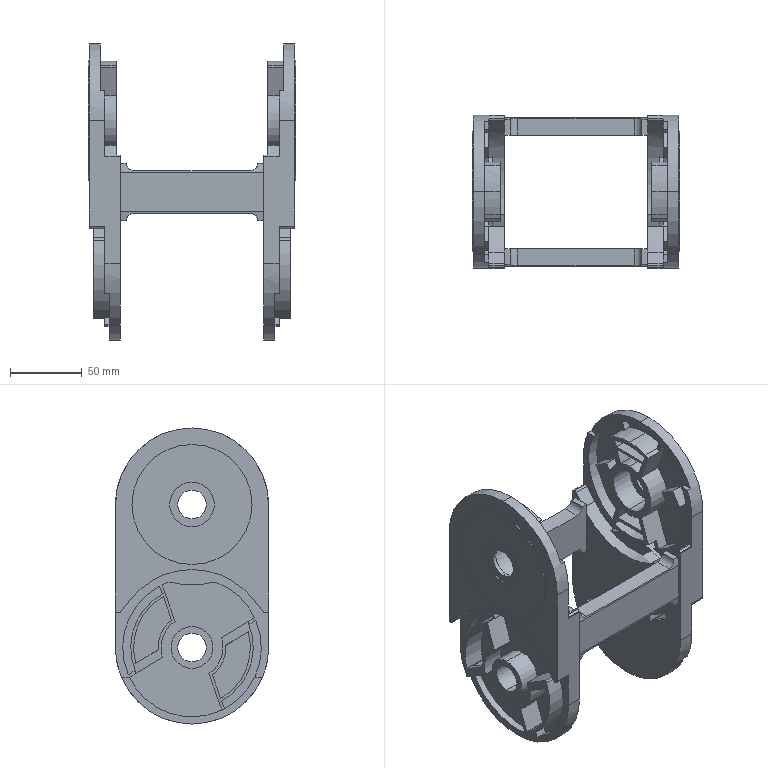Part | SolidWorks | features BaseBody 1 | 1 solid | 402 faces | box 145 x 107 x 206.999 mm | volume 368273 mm3 | plane 216 | cylinder 186 | commonest cylinder face diameters 97 x30 1 x12 4 x12 47.5 x12 81.7 x12 85.7 x12